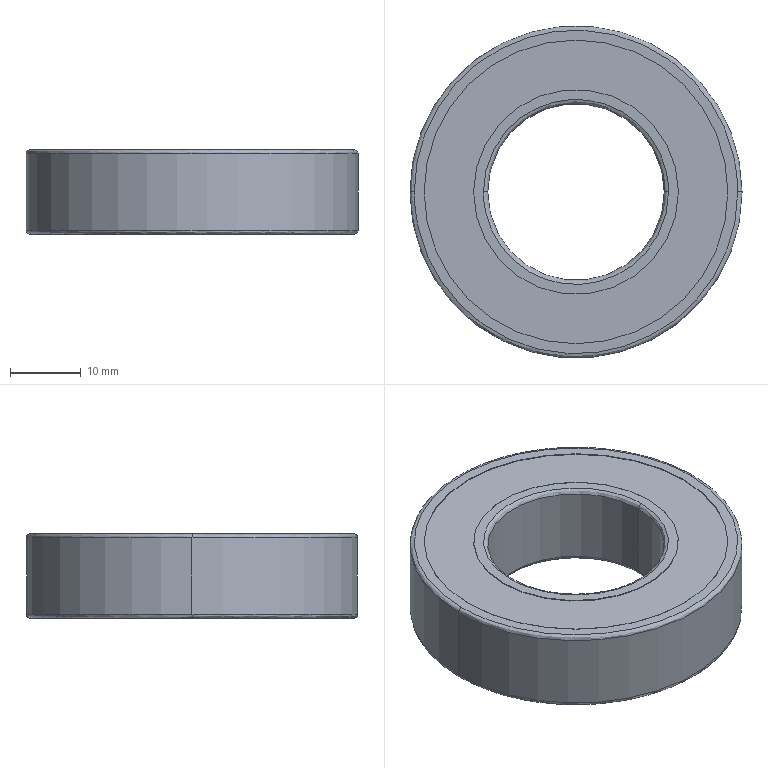Part | SolidWorks | features BaseBody 1 | 1 solid | 26 faces | box 47 x 47 x 12 mm | volume 14738 mm3 | cylinder 12 | spline 8 | plane 6 | commonest cylinder face diameters 29 x4 43 x4 25 x2 47 x2
STEP:
#1=CARTESIAN_POINT('',(-22.9,0.,-12.));
#2=VERTEX_POINT('',#1);
#3=CARTESIAN_POINT('',(22.9,0.,-12.));
#4=VERTEX_POINT('',#3);
#5=CARTESIAN_POINT('',(-22.9,0.,-12.));
#6=CARTESIAN_POINT('',(-22.9,-45.8,-12.));
#7=CARTESIAN_POINT('',(22.9,-45.8,-12.));
#8=CARTESIAN_POINT('',(22.9,0.,-12.));
#9=(BOUNDED_CURVE()B_SPLINE_CURVE(3,(#5,#6,#7,#8),.UNSPECIFIED.,.F.,.F.)B_SPLINE_CURVE_WITH_KNOTS((4,4),(0.,0.5),.UNSPECIFIED.)CURVE()GEOMETRIC_REPRESENTATION_ITEM()RATIONAL_B_SPLINE_CURVE((1.,0.3333,0.3333,1.))REPRESENTATION_ITEM(''));
#10=EDGE_CURVE('',#2,#4,#9,.T.);
#11=ORIENTED_EDGE('',*,*,#10,.T.);
#12=CARTESIAN_POINT('',(23.5,0.,-11.4));
#13=VERTEX_POINT('',#12);
#14=CARTESIAN_POINT('',(22.9,0.,-11.4));
#15=DIRECTION('',(0.,-1.,0.));
#16=DIRECTION('',(1.,0.,0.));
#17=AXIS2_PLACEMENT_3D('',#14,#15,#16);
#18=CIRCLE('',#17,0.6);
#19=EDGE_CURVE('',#4,#13,#18,.T.);
#20=ORIENTED_EDGE('',*,*,#19,.T.);
#21=CARTESIAN_POINT('',(-23.5,0.,-11.4));
#22=VERTEX_POINT('',#21);
#23=CARTESIAN_POINT('',(0.,0.,-11.4));
#24=DIRECTION('',(0.,0.,1.));
#25=DIRECTION('',(1.,0.,0.));
#26=AXIS2_PLACEMENT_3D('',#23,#24,#25);
#27=CIRCLE('',#26,23.5);
#28=EDGE_CURVE('',#22,#13,#27,.T.);
#29=ORIENTED_EDGE('',*,*,#28,.F.);
#30=CARTESIAN_POINT('',(-22.9,0.,-11.4));
#31=DIRECTION('',(0.,1.,0.));
#32=DIRECTION('',(-1.,0.,0.));
#33=AXIS2_PLACEMENT_3D('',#30,#31,#32);
#34=CIRCLE('',#33,0.6);
#35=EDGE_CURVE('',#2,#22,#34,.T.);
#36=ORIENTED_EDGE('',*,*,#35,.F.);
#37=EDGE_LOOP('',(#11,#20,#29,#36));
#38=FACE_OUTER_BOUND('',#37,.T.);
#39=CARTESIAN_POINT('',(22.9,0.,-12.));
#40=CARTESIAN_POINT('',(22.9,-45.8,-12.));
#41=CARTESIAN_POINT('',(-22.9,-45.8,-12.));
#42=CARTESIAN_POINT('',(-22.9,0.,-12.));
#43=CARTESIAN_POINT('',(23.251,0.,-12.));
#44=CARTESIAN_POINT('',(23.251,-46.503,-12.));
#45=CARTESIAN_POINT('',(-23.251,-46.503,-12.));
#46=CARTESIAN_POINT('',(-23.251,0.,-12.));
#47=CARTESIAN_POINT('',(23.5,0.,-11.751));
#48=CARTESIAN_POINT('',(23.5,-47.,-11.751));
#49=CARTESIAN_POINT('',(-23.5,-47.,-11.751));
#50=CARTESIAN_POINT('',(-23.5,0.,-11.751));
#51=CARTESIAN_POINT('',(23.5,0.,-11.4));
#52=CARTESIAN_POINT('',(23.5,-47.,-11.4));
#53=CARTESIAN_POINT('',(-23.5,-47.,-11.4));
#54=CARTESIAN_POINT('',(-23.5,0.,-11.4));
#55=(BOUNDED_SURFACE()B_SPLINE_SURFACE(3,3,((#39,#40,#41,#42),(#43,#44,#45,#46),(#47,#48,#49,#50),(#51,#52,#53,#54)),.UNSPECIFIED.,.F.,.F.,.F.)B_SPLINE_SURFACE_WITH_KNOTS((4,4),(4,4),(0.,1.),(0.,1.),.UNSPECIFIED.)GEOMETRIC_REPRESENTATION_ITEM()RATIONAL_B_SPLINE_SURFACE(((1.,0.3333,0.3333,1.),(0.8047,0.2682,0.2682,0.8047),(0.8047,0.2682,0.2682,0.8047),(1.,0.3333,0.3333,1.)))REPRESENTATION_ITEM('')SURFACE());
#56=ADVANCED_FACE('',(#38),#55,.T.);
#57=CARTESIAN_POINT('',(23.5,0.,-0.6));
#58=VERTEX_POINT('',#57);
#59=CARTESIAN_POINT('',(-23.5,0.,-0.6));
#60=VERTEX_POINT('',#59);
#61=CARTESIAN_POINT('',(0.,0.,-0.6));
#62=DIRECTION('',(0.,0.,-1.));
#63=DIRECTION('',(1.,0.,0.));
#64=AXIS2_PLACEMENT_3D('',#61,#62,#63);
#65=CIRCLE('',#64,23.5);
#66=EDGE_CURVE('',#58,#60,#65,.T.);
#67=ORIENTED_EDGE('',*,*,#66,.F.);
#68=CARTESIAN_POINT('',(22.9,0.,0.));
#69=VERTEX_POINT('',#68);
#70=CARTESIAN_POINT('',(22.9,0.,-0.6));
#71=DIRECTION('',(0.,-1.,0.));
#72=DIRECTION('',(1.,0.,0.));
#73=AXIS2_PLACEMENT_3D('',#70,#71,#72);
#74=CIRCLE('',#73,0.6);
#75=EDGE_CURVE('',#58,#69,#74,.T.);
#76=ORIENTED_EDGE('',*,*,#75,.T.);
#77=CARTESIAN_POINT('',(-22.9,0.,0.));
#78=VERTEX_POINT('',#77);
#79=CARTESIAN_POINT('',(22.9,0.,0.));
#80=CARTESIAN_POINT('',(22.9,-45.8,0.));
#81=CARTESIAN_POINT('',(-22.9,-45.8,0.));
#82=CARTESIAN_POINT('',(-22.9,0.,0.));
#83=(BOUNDED_CURVE()B_SPLINE_CURVE(3,(#79,#80,#81,#82),.UNSPECIFIED.,.F.,.F.)B_SPLINE_CURVE_WITH_KNOTS((4,4),(0.5,1.),.UNSPECIFIED.)CURVE()GEOMETRIC_REPRESENTATION_ITEM()RATIONAL_B_SPLINE_CURVE((1.,0.3333,0.3333,1.))REPRESENTATION_ITEM(''));
#84=EDGE_CURVE('',#69,#78,#83,.T.);
#85=ORIENTED_EDGE('',*,*,#84,.T.);
#86=CARTESIAN_POINT('',(-22.9,0.,-0.6));
#87=DIRECTION('',(0.,1.,0.));
#88=DIRECTION('',(-1.,0.,0.));
#89=AXIS2_PLACEMENT_3D('',#86,#87,#88);
#90=CIRCLE('',#89,0.6);
#91=EDGE_CURVE('',#60,#78,#90,.T.);
#92=ORIENTED_EDGE('',*,*,#91,.F.);
#93=EDGE_LOOP('',(#67,#76,#85,#92));
#94=FACE_OUTER_BOUND('',#93,.T.);
#95=CARTESIAN_POINT('',(23.5,0.,-0.6));
#96=CARTESIAN_POINT('',(23.5,-47.,-0.6));
#97=CARTESIAN_POINT('',(-23.5,-47.,-0.6));
#98=CARTESIAN_POINT('',(-23.5,0.,-0.6));
#99=CARTESIAN_POINT('',(23.5,0.,-0.2485));
#100=CARTESIAN_POINT('',(23.5,-47.,-0.2485));
#101=CARTESIAN_POINT('',(-23.5,-47.,-0.2485));
#102=CARTESIAN_POINT('',(-23.5,0.,-0.2485));
#103=CARTESIAN_POINT('',(23.251,0.,0.));
#104=CARTESIAN_POINT('',(23.251,-46.503,0.));
#105=CARTESIAN_POINT('',(-23.251,-46.503,0.));
#106=CARTESIAN_POINT('',(-23.251,0.,0.));
#107=CARTESIAN_POINT('',(22.9,0.,0.));
#108=CARTESIAN_POINT('',(22.9,-45.8,0.));
#109=CARTESIAN_POINT('',(-22.9,-45.8,0.));
#110=CARTESIAN_POINT('',(-22.9,0.,0.));
#111=(BOUNDED_SURFACE()B_SPLINE_SURFACE(3,3,((#95,#96,#97,#98),(#99,#100,#101,#102),(#103,#104,#105,#106),(#107,#108,#109,#110)),.UNSPECIFIED.,.F.,.F.,.F.)B_SPLINE_SURFACE_WITH_KNOTS((4,4),(4,4),(0.,1.),(0.,1.),.UNSPECIFIED.)GEOMETRIC_REPRESENTATION_ITEM()RATIONAL_B_SPLINE_SURFACE(((1.,0.3333,0.3333,1.),(0.8047,0.2682,0.2682,0.8047),(0.8047,0.2682,0.2682,0.8047),(1.,0.3333,0.3333,1.)))REPRESENTATION_ITEM('')SURFACE());
#112=ADVANCED_FACE('',(#94),#111,.T.);
#113=CARTESIAN_POINT('',(-12.5,0.,-11.4));
#114=VERTEX_POINT('',#113);
#115=CARTESIAN_POINT('',(12.5,0.,-11.4));
#116=VERTEX_POINT('',#115);
#117=CARTESIAN_POINT('',(0.,0.,-11.4));
#118=DIRECTION('',(0.,0.,1.));
#119=DIRECTION('',(-1.,0.,0.));
#120=AXIS2_PLACEMENT_3D('',#117,#118,#119);
#121=CIRCLE('',#120,12.5);
#122=EDGE_CURVE('',#114,#116,#121,.T.);
#123=ORIENTED_EDGE('',*,*,#122,.T.);
#124=CARTESIAN_POINT('',(13.1,0.,-12.));
#125=VERTEX_POINT('',#124);
#126=CARTESIAN_POINT('',(13.1,0.,-11.4));
#127=DIRECTION('',(0.,-1.,0.));
#128=DIRECTION('',(1.,0.,0.));
#129=AXIS2_PLACEMENT_3D('',#126,#127,#128);
#130=CIRCLE('',#129,0.6);
#131=EDGE_CURVE('',#116,#125,#130,.T.);
#132=ORIENTED_EDGE('',*,*,#131,.T.);
#133=CARTESIAN_POINT('',(-13.1,0.,-12.));
#134=VERTEX_POINT('',#133);
#135=CARTESIAN_POINT('',(-13.1,0.,-12.));
#136=CARTESIAN_POINT('',(-13.1,-0.4005,-12.));
#137=CARTESIAN_POINT('',(-13.073,-0.9989,-12.));
#138=CARTESIAN_POINT('',(-12.993,-1.693,-12.));
#139=CARTESIAN_POINT('',(-12.941,-2.039,-12.));
#140=CARTESIAN_POINT('',(-12.912,-2.211,-12.));
#141=CARTESIAN_POINT('',(-12.899,-2.285,-12.));
#142=CARTESIAN_POINT('',(-12.89,-2.334,-12.));
#143=CARTESIAN_POINT('',(-12.886,-2.358,-12.));
#144=CARTESIAN_POINT('',(-12.804,-2.801,-12.));
#145=CARTESIAN_POINT('',(-12.658,-3.419,-12.));
#146=CARTESIAN_POINT('',(-12.437,-4.126,-12.));
#147=CARTESIAN_POINT('',(-12.313,-4.475,-12.));
#148=CARTESIAN_POINT('',(-12.257,-4.624,-12.));
#149=CARTESIAN_POINT('',(-12.219,-4.723,-12.));
#150=CARTESIAN_POINT('',(-12.201,-4.771,-12.));
#151=CARTESIAN_POINT('',(-12.017,-5.233,-12.));
#152=CARTESIAN_POINT('',(-11.743,-5.835,-12.));
#153=CARTESIAN_POINT('',(-11.371,-6.511,-12.));
#154=CARTESIAN_POINT('',(-11.172,-6.842,-12.));
#155=CARTESIAN_POINT('',(-11.084,-6.982,-12.));
#156=CARTESIAN_POINT('',(-11.025,-7.076,-12.));
#157=CARTESIAN_POINT('',(-10.996,-7.121,-12.));
#158=CARTESIAN_POINT('',(-10.47,-7.925,-12.));
#159=CARTESIAN_POINT('',(-9.902,-8.624,-12.));
#160=CARTESIAN_POINT('',(-8.943,-9.583,-12.));
#161=CARTESIAN_POINT('',(-8.442,-10.035,-12.));
#162=CARTESIAN_POINT('',(-7.818,-10.516,-12.));
#163=CARTESIAN_POINT('',(-7.497,-10.744,-12.));
#164=CARTESIAN_POINT('',(-7.357,-10.839,-12.));
#165=CARTESIAN_POINT('',(-7.263,-10.902,-12.));
#166=CARTESIAN_POINT('',(-7.215,-10.934,-12.));
#167=CARTESIAN_POINT('',(-6.798,-11.207,-12.));
#168=CARTESIAN_POINT('',(-6.227,-11.54,-12.));
#169=CARTESIAN_POINT('',(-5.534,-11.878,-12.));
#170=CARTESIAN_POINT('',(-5.18,-12.033,-12.));
#171=CARTESIAN_POINT('',(-5.002,-12.108,-12.));
#172=CARTESIAN_POINT('',(-4.925,-12.139,-12.));
#173=CARTESIAN_POINT('',(-4.873,-12.16,-12.));
#174=CARTESIAN_POINT('',(-4.847,-12.17,-12.));
#175=CARTESIAN_POINT('',(-4.427,-12.337,-12.));
#176=CARTESIAN_POINT('',(-3.826,-12.541,-12.));
#177=CARTESIAN_POINT('',(-3.11,-12.729,-12.));
#178=CARTESIAN_POINT('',(-2.748,-12.809,-12.));
#179=CARTESIAN_POINT('',(-2.566,-12.846,-12.));
#180=CARTESIAN_POINT('',(-2.488,-12.862,-12.));
#181=CARTESIAN_POINT('',(-2.436,-12.872,-12.));
#182=CARTESIAN_POINT('',(-2.408,-12.877,-12.));
#183=CARTESIAN_POINT('',(-1.596,-13.027,-12.));
#184=CARTESIAN_POINT('',(-0.8009,-13.1,-12.));
#185=CARTESIAN_POINT('',(0.4005,-13.1,-12.));
#186=CARTESIAN_POINT('',(0.9988,-13.073,-12.));
#187=CARTESIAN_POINT('',(1.693,-12.993,-12.));
#188=CARTESIAN_POINT('',(2.039,-12.941,-12.));
#189=CARTESIAN_POINT('',(2.211,-12.912,-12.));
#190=CARTESIAN_POINT('',(2.285,-12.899,-12.));
#191=CARTESIAN_POINT('',(2.334,-12.89,-12.));
#192=CARTESIAN_POINT('',(2.358,-12.886,-12.));
#193=CARTESIAN_POINT('',(2.801,-12.804,-12.));
#194=CARTESIAN_POINT('',(3.419,-12.658,-12.));
#195=CARTESIAN_POINT('',(4.126,-12.437,-12.));
#196=CARTESIAN_POINT('',(4.475,-12.313,-12.));
#197=CARTESIAN_POINT('',(4.624,-12.257,-12.));
#198=CARTESIAN_POINT('',(4.723,-12.219,-12.));
#199=CARTESIAN_POINT('',(4.771,-12.201,-12.));
#200=CARTESIAN_POINT('',(5.233,-12.017,-12.));
#201=CARTESIAN_POINT('',(5.835,-11.743,-12.));
#202=CARTESIAN_POINT('',(6.511,-11.371,-12.));
#203=CARTESIAN_POINT('',(6.842,-11.172,-12.));
#204=CARTESIAN_POINT('',(6.982,-11.084,-12.));
#205=CARTESIAN_POINT('',(7.076,-11.025,-12.));
#206=CARTESIAN_POINT('',(7.121,-10.996,-12.));
#207=CARTESIAN_POINT('',(7.925,-10.47,-12.));
#208=CARTESIAN_POINT('',(8.624,-9.902,-12.));
#209=CARTESIAN_POINT('',(9.583,-8.943,-12.));
#210=CARTESIAN_POINT('',(10.035,-8.442,-12.));
#211=CARTESIAN_POINT('',(10.516,-7.818,-12.));
#212=CARTESIAN_POINT('',(10.744,-7.497,-12.));
#213=CARTESIAN_POINT('',(10.839,-7.357,-12.));
#214=CARTESIAN_POINT('',(10.902,-7.263,-12.));
#215=CARTESIAN_POINT('',(10.934,-7.215,-12.));
#216=CARTESIAN_POINT('',(11.207,-6.798,-12.));
#217=CARTESIAN_POINT('',(11.54,-6.227,-12.));
#218=CARTESIAN_POINT('',(11.878,-5.534,-12.));
#219=CARTESIAN_POINT('',(12.033,-5.18,-12.));
#220=CARTESIAN_POINT('',(12.108,-5.002,-12.));
#221=CARTESIAN_POINT('',(12.139,-4.925,-12.));
#222=CARTESIAN_POINT('',(12.16,-4.873,-12.));
#223=CARTESIAN_POINT('',(12.17,-4.847,-12.));
#224=CARTESIAN_POINT('',(12.337,-4.427,-12.));
#225=CARTESIAN_POINT('',(12.541,-3.826,-12.));
#226=CARTESIAN_POINT('',(12.729,-3.11,-12.));
#227=CARTESIAN_POINT('',(12.809,-2.748,-12.));
#228=CARTESIAN_POINT('',(12.846,-2.566,-12.));
#229=CARTESIAN_POINT('',(12.862,-2.488,-12.));
#230=CARTESIAN_POINT('',(12.872,-2.436,-12.));
#231=CARTESIAN_POINT('',(12.877,-2.408,-12.));
#232=CARTESIAN_POINT('',(13.027,-1.596,-12.));
#233=CARTESIAN_POINT('',(13.1,-0.8009,-12.));
#234=CARTESIAN_POINT('',(13.1,0.,-12.));
#235=B_SPLINE_CURVE_WITH_KNOTS('',3,(#135,#136,#137,#138,#139,#140,#141,#142,#143,#144,#145,#146,#147,#148,#149,#150,#151,#152,#153,#154,#155,#156,#157,#158,#159,#160,#161,#162,#163,#164,#165,#166,#167,#168,#169,#170,#171,#172,#173,#174,#175,#176,#177,#178,#179,#180,#181,#182,#183,#184,#185,#186,#187,#188,#189,#190,#191,#192,#193,#194,#195,#196,#197,#198,#199,#200,#201,#202,#203,#204,#205,#206,#207,#208,#209,#210,#211,#212,#213,#214,#215,#216,#217,#218,#219,#220,#221,#222,#223,#224,#225,#226,#227,#228,#229,#230,#231,#232,#233,#234),.UNSPECIFIED.,.F.,.F.,(4,1,1,1,1,2,2,1,1,1,2,2,1,1,1,2,2,2,1,1,1,2,2,1,1,1,1,2,2,1,1,1,1,2,2,2,1,1,1,1,2,2,1,1,1,2,2,1,1,1,2,2,2,1,1,1,2,2,1,1,1,1,2,2,1,1,1,1,2,2,4),(0.,0.01563,0.02344,0.02734,0.0293,0.03027,0.03125,0.04688,0.05469,0.05859,0.06055,0.0625,0.07813,0.08594,0.08984,0.0918,0.09375,0.125,0.1406,0.1484,0.1523,0.1543,0.1563,0.1719,0.1797,0.1836,0.1855,0.1865,0.1875,0.2031,0.2109,0.2148,0.2168,0.2178,0.2188,0.25,0.2656,0.2734,0.2773,0.2793,0.2803,0.2813,0.2969,0.3047,0.3086,0.3105,0.3125,0.3281,0.3359,0.3398,0.3418,0.3438,0.375,0.3906,0.3984,0.4023,0.4043,0.4063,0.4219,0.4297,0.4336,0.4355,0.4365,0.4375,0.4531,0.4609,0.4648,0.4668,0.4678,0.4688,0.5),.UNSPECIFIED.);
#236=EDGE_CURVE('',#134,#125,#235,.T.);
#237=ORIENTED_EDGE('',*,*,#236,.F.);
#238=CARTESIAN_POINT('',(-13.1,0.,-11.4));
#239=DIRECTION('',(0.,1.,0.));
#240=DIRECTION('',(-1.,0.,0.));
#241=AXIS2_PLACEMENT_3D('',#238,#239,#240);
#242=CIRCLE('',#241,0.6);
#243=EDGE_CURVE('',#114,#134,#242,.T.);
#244=ORIENTED_EDGE('',*,*,#243,.F.);
#245=EDGE_LOOP('',(#123,#132,#237,#244));
#246=FACE_OUTER_BOUND('',#245,.T.);
#247=CARTESIAN_POINT('',(12.5,0.,-11.4));
#248=CARTESIAN_POINT('',(12.5,-25.,-11.4));
#249=CARTESIAN_POINT('',(-12.5,-25.,-11.4));
#250=CARTESIAN_POINT('',(-12.5,0.,-11.4));
#251=CARTESIAN_POINT('',(12.5,0.,-11.751));
#252=CARTESIAN_POINT('',(12.5,-25.,-11.751));
#253=CARTESIAN_POINT('',(-12.5,-25.,-11.751));
#254=CARTESIAN_POINT('',(-12.5,0.,-11.751));
#255=CARTESIAN_POINT('',(12.749,0.,-12.));
#256=CARTESIAN_POINT('',(12.749,-25.497,-12.));
#257=CARTESIAN_POINT('',(-12.749,-25.497,-12.));
#258=CARTESIAN_POINT('',(-12.749,0.,-12.));
#259=CARTESIAN_POINT('',(13.1,0.,-12.));
#260=CARTESIAN_POINT('',(13.1,-26.2,-12.));
#261=CARTESIAN_POINT('',(-13.1,-26.2,-12.));
#262=CARTESIAN_POINT('',(-13.1,0.,-12.));
#263=(BOUNDED_SURFACE()B_SPLINE_SURFACE(3,3,((#247,#248,#249,#250),(#251,#252,#253,#254),(#255,#256,#257,#258),(#259,#260,#261,#262)),.UNSPECIFIED.,.F.,.F.,.F.)B_SPLINE_SURFACE_WITH_KNOTS((4,4),(4,4),(0.,1.),(0.,1.),.UNSPECIFIED.)GEOMETRIC_REPRESENTATION_ITEM()RATIONAL_B_SPLINE_SURFACE(((1.,0.3333,0.3333,1.),(0.8047,0.2682,0.2682,0.8047),(0.8047,0.2682,0.2682,0.8047),(1.,0.3333,0.3333,1.)))REPRESENTATION_ITEM('')SURFACE());
#264=ADVANCED_FACE('',(#246),#263,.T.);
#265=CARTESIAN_POINT('',(13.1,0.,0.));
#266=VERTEX_POINT('',#265);
#267=CARTESIAN_POINT('',(-13.1,0.,0.));
#268=VERTEX_POINT('',#267);
#269=CARTESIAN_POINT('',(13.1,0.,0.));
#270=CARTESIAN_POINT('',(13.1,-0.4005,0.));
#271=CARTESIAN_POINT('',(13.073,-0.9988,0.));
#272=CARTESIAN_POINT('',(12.993,-1.693,0.));
#273=CARTESIAN_POINT('',(12.941,-2.039,0.));
#274=CARTESIAN_POINT('',(12.912,-2.211,0.));
#275=CARTESIAN_POINT('',(12.899,-2.285,0.));
#276=CARTESIAN_POINT('',(12.89,-2.334,0.));
#277=CARTESIAN_POINT('',(12.886,-2.358,0.));
#278=CARTESIAN_POINT('',(12.804,-2.801,0.));
#279=CARTESIAN_POINT('',(12.658,-3.419,0.));
#280=CARTESIAN_POINT('',(12.437,-4.126,0.));
#281=CARTESIAN_POINT('',(12.313,-4.475,0.));
#282=CARTESIAN_POINT('',(12.257,-4.624,0.));
#283=CARTESIAN_POINT('',(12.219,-4.723,0.));
#284=CARTESIAN_POINT('',(12.201,-4.771,0.));
#285=CARTESIAN_POINT('',(12.017,-5.233,0.));
#286=CARTESIAN_POINT('',(11.743,-5.835,0.));
#287=CARTESIAN_POINT('',(11.371,-6.511,0.));
#288=CARTESIAN_POINT('',(11.172,-6.842,0.));
#289=CARTESIAN_POINT('',(11.084,-6.982,0.));
#290=CARTESIAN_POINT('',(11.025,-7.076,0.));
#291=CARTESIAN_POINT('',(10.996,-7.121,0.));
#292=CARTESIAN_POINT('',(10.47,-7.925,0.));
#293=CARTESIAN_POINT('',(9.902,-8.624,0.));
#294=CARTESIAN_POINT('',(8.943,-9.583,0.));
#295=CARTESIAN_POINT('',(8.442,-10.035,0.));
#296=CARTESIAN_POINT('',(7.818,-10.516,0.));
#297=CARTESIAN_POINT('',(7.497,-10.744,0.));
#298=CARTESIAN_POINT('',(7.357,-10.839,0.));
#299=CARTESIAN_POINT('',(7.263,-10.902,0.));
#300=CARTESIAN_POINT('',(7.215,-10.934,0.));
#301=CARTESIAN_POINT('',(6.798,-11.207,0.));
#302=CARTESIAN_POINT('',(6.227,-11.54,0.));
#303=CARTESIAN_POINT('',(5.534,-11.878,0.));
#304=CARTESIAN_POINT('',(5.18,-12.033,0.));
#305=CARTESIAN_POINT('',(5.002,-12.108,0.));
#306=CARTESIAN_POINT('',(4.925,-12.139,0.));
#307=CARTESIAN_POINT('',(4.873,-12.16,0.));
#308=CARTESIAN_POINT('',(4.847,-12.17,0.));
#309=CARTESIAN_POINT('',(4.427,-12.337,0.));
#310=CARTESIAN_POINT('',(3.826,-12.541,0.));
#311=CARTESIAN_POINT('',(3.11,-12.729,0.));
#312=CARTESIAN_POINT('',(2.748,-12.809,0.));
#313=CARTESIAN_POINT('',(2.566,-12.846,0.));
#314=CARTESIAN_POINT('',(2.488,-12.862,0.));
#315=CARTESIAN_POINT('',(2.436,-12.872,0.));
#316=CARTESIAN_POINT('',(2.408,-12.877,0.));
#317=CARTESIAN_POINT('',(1.596,-13.027,0.));
#318=CARTESIAN_POINT('',(0.8009,-13.1,0.));
#319=CARTESIAN_POINT('',(-0.4005,-13.1,0.));
#320=CARTESIAN_POINT('',(-0.9988,-13.073,0.));
#321=CARTESIAN_POINT('',(-1.693,-12.993,0.));
#322=CARTESIAN_POINT('',(-2.039,-12.941,0.));
#323=CARTESIAN_POINT('',(-2.211,-12.912,0.));
#324=CARTESIAN_POINT('',(-2.285,-12.899,0.));
#325=CARTESIAN_POINT('',(-2.334,-12.89,0.));
#326=CARTESIAN_POINT('',(-2.358,-12.886,0.));
#327=CARTESIAN_POINT('',(-2.801,-12.804,0.));
#328=CARTESIAN_POINT('',(-3.419,-12.658,0.));
#329=CARTESIAN_POINT('',(-4.126,-12.437,0.));
#330=CARTESIAN_POINT('',(-4.475,-12.313,0.));
#331=CARTESIAN_POINT('',(-4.624,-12.257,0.));
#332=CARTESIAN_POINT('',(-4.723,-12.219,0.));
#333=CARTESIAN_POINT('',(-4.771,-12.201,0.));
#334=CARTESIAN_POINT('',(-5.233,-12.017,0.));
#335=CARTESIAN_POINT('',(-5.835,-11.743,0.));
#336=CARTESIAN_POINT('',(-6.511,-11.371,0.));
#337=CARTESIAN_POINT('',(-6.842,-11.172,0.));
#338=CARTESIAN_POINT('',(-6.982,-11.084,0.));
#339=CARTESIAN_POINT('',(-7.076,-11.025,0.));
#340=CARTESIAN_POINT('',(-7.121,-10.996,0.));
#341=CARTESIAN_POINT('',(-7.925,-10.47,0.));
#342=CARTESIAN_POINT('',(-8.624,-9.902,0.));
#343=CARTESIAN_POINT('',(-9.583,-8.943,0.));
#344=CARTESIAN_POINT('',(-10.035,-8.442,0.));
#345=CARTESIAN_POINT('',(-10.516,-7.818,0.));
#346=CARTESIAN_POINT('',(-10.744,-7.497,0.));
#347=CARTESIAN_POINT('',(-10.839,-7.357,0.));
#348=CARTESIAN_POINT('',(-10.902,-7.263,0.));
#349=CARTESIAN_POINT('',(-10.934,-7.215,0.));
#350=CARTESIAN_POINT('',(-11.207,-6.798,0.));
#351=CARTESIAN_POINT('',(-11.54,-6.227,0.));
#352=CARTESIAN_POINT('',(-11.878,-5.534,0.));
#353=CARTESIAN_POINT('',(-12.033,-5.18,0.));
#354=CARTESIAN_POINT('',(-12.108,-5.002,0.));
#355=CARTESIAN_POINT('',(-12.139,-4.925,0.));
#356=CARTESIAN_POINT('',(-12.16,-4.873,0.));
#357=CARTESIAN_POINT('',(-12.17,-4.847,0.));
#358=CARTESIAN_POINT('',(-12.337,-4.427,0.));
#359=CARTESIAN_POINT('',(-12.541,-3.826,0.));
#360=CARTESIAN_POINT('',(-12.729,-3.11,0.));
#361=CARTESIAN_POINT('',(-12.809,-2.748,0.));
#362=CARTESIAN_POINT('',(-12.846,-2.566,0.));
#363=CARTESIAN_POINT('',(-12.862,-2.488,0.));
#364=CARTESIAN_POINT('',(-12.872,-2.436,0.));
#365=CARTESIAN_POINT('',(-12.877,-2.408,0.));
#366=CARTESIAN_POINT('',(-13.027,-1.596,0.));
#367=CARTESIAN_POINT('',(-13.1,-0.8014,0.));
#368=CARTESIAN_POINT('',(-13.1,0.,0.));
#369=B_SPLINE_CURVE_WITH_KNOTS('',3,(#269,#270,#271,#272,#273,#274,#275,#276,#277,#278,#279,#280,#281,#282,#283,#284,#285,#286,#287,#288,#289,#290,#291,#292,#293,#294,#295,#296,#297,#298,#299,#300,#301,#302,#303,#304,#305,#306,#307,#308,#309,#310,#311,#312,#313,#314,#315,#316,#317,#318,#319,#320,#321,#322,#323,#324,#325,#326,#327,#328,#329,#330,#331,#332,#333,#334,#335,#336,#337,#338,#339,#340,#341,#342,#343,#344,#345,#346,#347,#348,#349,#350,#351,#352,#353,#354,#355,#356,#357,#358,#359,#360,#361,#362,#363,#364,#365,#366,#367,#368),.UNSPECIFIED.,.F.,.F.,(4,1,1,1,1,2,2,1,1,1,2,2,1,1,1,2,2,2,1,1,1,2,2,1,1,1,1,2,2,1,1,1,1,2,2,2,1,1,1,1,2,2,1,1,1,2,2,1,1,1,2,2,2,1,1,1,2,2,1,1,1,1,2,2,1,1,1,1,2,2,4),(0.5,0.5156,0.5234,0.5273,0.5293,0.5303,0.5313,0.5469,0.5547,0.5586,0.5605,0.5625,0.5781,0.5859,0.5898,0.5918,0.5938,0.625,0.6406,0.6484,0.6523,0.6543,0.6563,0.6719,0.6797,0.6836,0.6855,0.6865,0.6875,0.7031,0.7109,0.7148,0.7168,0.7178,0.7188,0.75,0.7656,0.7734,0.7773,0.7793,0.7803,0.7813,0.7969,0.8047,0.8086,0.8105,0.8125,0.8281,0.8359,0.8398,0.8418,0.8438,0.875,0.8906,0.8984,0.9023,0.9043,0.9062,0.9219,0.9297,0.9336,0.9355,0.9365,0.9375,0.9531,0.9609,0.9648,0.9668,0.9678,0.9687,1.),.UNSPECIFIED.);
#370=EDGE_CURVE('',#266,#268,#369,.T.);
#371=ORIENTED_EDGE('',*,*,#370,.F.);
#372=CARTESIAN_POINT('',(12.5,0.,-0.6));
#373=VERTEX_POINT('',#372);
#374=CARTESIAN_POINT('',(13.1,0.,-0.6));
#375=DIRECTION('',(0.,-1.,0.));
#376=DIRECTION('',(1.,0.,0.));
#377=AXIS2_PLACEMENT_3D('',#374,#375,#376);
#378=CIRCLE('',#377,0.6);
#379=EDGE_CURVE('',#266,#373,#378,.T.);
#380=ORIENTED_EDGE('',*,*,#379,.T.);
#381=CARTESIAN_POINT('',(-12.5,0.,-0.6));
#382=VERTEX_POINT('',#381);
#383=CARTESIAN_POINT('',(0.,0.,-0.6));
#384=DIRECTION('',(0.,0.,-1.));
#385=DIRECTION('',(-1.,0.,0.));
#386=AXIS2_PLACEMENT_3D('',#383,#384,#385);
#387=CIRCLE('',#386,12.5);
#388=EDGE_CURVE('',#373,#382,#387,.T.);
#389=ORIENTED_EDGE('',*,*,#388,.T.);
#390=CARTESIAN_POINT('',(-13.1,0.,-0.6));
#391=DIRECTION('',(0.,1.,0.));
#392=DIRECTION('',(-1.,0.,0.));
#393=AXIS2_PLACEMENT_3D('',#390,#391,#392);
#394=CIRCLE('',#393,0.6);
#395=EDGE_CURVE('',#268,#382,#394,.T.);
#396=ORIENTED_EDGE('',*,*,#395,.F.);
#397=EDGE_LOOP('',(#371,#380,#389,#396));
#398=FACE_OUTER_BOUND('',#397,.T.);
#399=CARTESIAN_POINT('',(13.1,0.,0.));
#400=CARTESIAN_POINT('',(13.1,-26.2,0.));
#401=CARTESIAN_POINT('',(-13.1,-26.2,0.));
#402=CARTESIAN_POINT('',(-13.1,0.,0.));
#403=CARTESIAN_POINT('',(12.749,0.,0.));
#404=CARTESIAN_POINT('',(12.749,-25.497,0.));
#405=CARTESIAN_POINT('',(-12.749,-25.497,0.));
#406=CARTESIAN_POINT('',(-12.749,0.,0.));
#407=CARTESIAN_POINT('',(12.5,0.,-0.2485));
#408=CARTESIAN_POINT('',(12.5,-25.,-0.2485));
#409=CARTESIAN_POINT('',(-12.5,-25.,-0.2485));
#410=CARTESIAN_POINT('',(-12.5,0.,-0.2485));
#411=CARTESIAN_POINT('',(12.5,0.,-0.6));
#412=CARTESIAN_POINT('',(12.5,-25.,-0.6));
#413=CARTESIAN_POINT('',(-12.5,-25.,-0.6));
#414=CARTESIAN_POINT('',(-12.5,0.,-0.6));
#415=(BOUNDED_SURFACE()B_SPLINE_SURFACE(3,3,((#399,#400,#401,#402),(#403,#404,#405,#406),(#407,#408,#409,#410),(#411,#412,#413,#414)),.UNSPECIFIED.,.F.,.F.,.F.)B_SPLINE_SURFACE_WITH_KNOTS((4,4),(4,4),(0.,1.),(0.,1.),.UNSPECIFIED.)GEOMETRIC_REPRESENTATION_ITEM()RATIONAL_B_SPLINE_SURFACE(((1.,0.3333,0.3333,1.),(0.8047,0.2682,0.2682,0.8047),(0.8047,0.2682,0.2682,0.8047),(1.,0.3333,0.3333,1.)))REPRESENTATION_ITEM('')SURFACE());
#416=ADVANCED_FACE('',(#398),#415,.T.);
#417=CARTESIAN_POINT('',(0.,0.,-11.4));
#418=DIRECTION('',(0.,0.,1.));
#419=DIRECTION('',(1.,0.,0.));
#420=AXIS2_PLACEMENT_3D('',#417,#418,#419);
#421=CIRCLE('',#420,23.5);
#422=EDGE_CURVE('',#13,#22,#421,.T.);
#423=ORIENTED_EDGE('',*,*,#422,.T.);
#424=CARTESIAN_POINT('',(-23.5,0.,-12.));
#425=DIRECTION('',(0.,0.,1.));
#426=VECTOR('',#425,1000.);
#427=LINE('',#424,#426);
#428=EDGE_CURVE('',#22,#60,#427,.T.);
#429=ORIENTED_EDGE('',*,*,#428,.T.);
#430=CARTESIAN_POINT('',(0.,0.,-0.6));
#431=DIRECTION('',(0.,0.,-1.));
#432=DIRECTION('',(1.,0.,0.));
#433=AXIS2_PLACEMENT_3D('',#430,#431,#432);
#434=CIRCLE('',#433,23.5);
#435=EDGE_CURVE('',#60,#58,#434,.T.);
#436=ORIENTED_EDGE('',*,*,#435,.T.);
#437=CARTESIAN_POINT('',(23.5,0.,-12.));
#438=DIRECTION('',(0.,0.,1.));
#439=VECTOR('',#438,1000.);
#440=LINE('',#437,#439);
#441=EDGE_CURVE('',#13,#58,#440,.T.);
#442=ORIENTED_EDGE('',*,*,#441,.F.);
#443=EDGE_LOOP('',(#423,#429,#436,#442));
#444=FACE_OUTER_BOUND('',#443,.T.);
#445=CARTESIAN_POINT('',(0.,0.,-12.));
#446=DIRECTION('',(0.,0.,1.));
#447=DIRECTION('',(1.,0.,0.));
#448=AXIS2_PLACEMENT_3D('',#445,#446,#447);
#449=CYLINDRICAL_SURFACE('',#448,23.5);
#450=ADVANCED_FACE('',(#444),#449,.T.);
#451=CARTESIAN_POINT('',(-21.5,0.,-12.));
#452=VERTEX_POINT('',#451);
#453=CARTESIAN_POINT('',(21.5,0.,-12.));
#454=VERTEX_POINT('',#453);
#455=CARTESIAN_POINT('',(0.,0.,-12.));
#456=DIRECTION('',(0.,0.,1.));
#457=DIRECTION('',(1.,0.,0.));
#458=AXIS2_PLACEMENT_3D('',#455,#456,#457);
#459=CIRCLE('',#458,21.5);
#460=EDGE_CURVE('',#452,#454,#459,.T.);
#461=ORIENTED_EDGE('',*,*,#460,.F.);
#462=CARTESIAN_POINT('',(-21.5,0.,-11.9));
#463=VERTEX_POINT('',#462);
#464=CARTESIAN_POINT('',(-21.5,0.,-12.));
#465=DIRECTION('',(0.,0.,1.));
#466=VECTOR('',#465,1000.);
#467=LINE('',#464,#466);
#468=EDGE_CURVE('',#452,#463,#467,.T.);
#469=ORIENTED_EDGE('',*,*,#468,.T.);
#470=CARTESIAN_POINT('',(21.5,0.,-11.9));
#471=VERTEX_POINT('',#470);
#472=CARTESIAN_POINT('',(0.,0.,-11.9));
#473=DIRECTION('',(0.,0.,-1.));
#474=DIRECTION('',(1.,0.,0.));
#475=AXIS2_PLACEMENT_3D('',#472,#473,#474);
#476=CIRCLE('',#475,21.5);
#477=EDGE_CURVE('',#471,#463,#476,.T.);
#478=ORIENTED_EDGE('',*,*,#477,.F.);
#479=CARTESIAN_POINT('',(21.5,0.,-12.));
#480=DIRECTION('',(0.,0.,1.));
#481=VECTOR('',#480,1000.);
#482=LINE('',#479,#481);
#483=EDGE_CURVE('',#454,#471,#482,.T.);
#484=ORIENTED_EDGE('',*,*,#483,.F.);
#485=EDGE_LOOP('',(#461,#469,#478,#484));
#486=FACE_OUTER_BOUND('',#485,.T.);
#487=CARTESIAN_POINT('',(0.,0.,-12.));
#488=DIRECTION('',(0.,0.,1.));
#489=DIRECTION('',(1.,0.,0.));
#490=AXIS2_PLACEMENT_3D('',#487,#488,#489);
#491=CYLINDRICAL_SURFACE('',#490,21.5);
#492=ADVANCED_FACE('',(#486),#491,.F.);
#493=CARTESIAN_POINT('',(-21.5,0.,-0.1));
#494=VERTEX_POINT('',#493);
#495=CARTESIAN_POINT('',(21.5,0.,-0.1));
#496=VERTEX_POINT('',#495);
#497=CARTESIAN_POINT('',(0.,0.,-0.1));
#498=DIRECTION('',(0.,0.,1.));
#499=DIRECTION('',(1.,0.,0.));
#500=AXIS2_PLACEMENT_3D('',#497,#498,#499);
#501=CIRCLE('',#500,21.5);
#502=EDGE_CURVE('',#494,#496,#501,.T.);
#503=ORIENTED_EDGE('',*,*,#502,.F.);
#504=CARTESIAN_POINT('',(-21.5,0.,0.));
#505=VERTEX_POINT('',#504);
#506=CARTESIAN_POINT('',(-21.5,0.,-12.));
#507=DIRECTION('',(0.,0.,1.));
#508=VECTOR('',#507,1000.);
#509=LINE('',#506,#508);
#510=EDGE_CURVE('',#494,#505,#509,.T.);
#511=ORIENTED_EDGE('',*,*,#510,.T.);
#512=CARTESIAN_POINT('',(21.5,0.,0.));
#513=VERTEX_POINT('',#512);
#514=CARTESIAN_POINT('',(0.,0.,0.));
#515=DIRECTION('',(0.,0.,-1.));
#516=DIRECTION('',(1.,0.,0.));
#517=AXIS2_PLACEMENT_3D('',#514,#515,#516);
#518=CIRCLE('',#517,21.5);
#519=EDGE_CURVE('',#513,#505,#518,.T.);
#520=ORIENTED_EDGE('',*,*,#519,.F.);
#521=CARTESIAN_POINT('',(21.5,0.,-12.));
#522=DIRECTION('',(0.,0.,1.));
#523=VECTOR('',#522,1000.);
#524=LINE('',#521,#523);
#525=EDGE_CURVE('',#496,#513,#524,.T.);
#526=ORIENTED_EDGE('',*,*,#525,.F.);
#527=EDGE_LOOP('',(#503,#511,#520,#526));
#528=FACE_OUTER_BOUND('',#527,.T.);
#529=CARTESIAN_POINT('',(0.,0.,-12.));
#530=DIRECTION('',(0.,0.,1.));
#531=DIRECTION('',(1.,0.,0.));
#532=AXIS2_PLACEMENT_3D('',#529,#530,#531);
#533=CYLINDRICAL_SURFACE('',#532,21.5);
#534=ADVANCED_FACE('',(#528),#533,.F.);
#535=CARTESIAN_POINT('',(14.5,0.,-12.));
#536=VERTEX_POINT('',#535);
#537=CARTESIAN_POINT('',(-14.5,0.,-12.));
#538=VERTEX_POINT('',#537);
#539=CARTESIAN_POINT('',(0.,0.,-12.));
#540=DIRECTION('',(0.,0.,1.));
#541=DIRECTION('',(1.,0.,0.));
#542=AXIS2_PLACEMENT_3D('',#539,#540,#541);
#543=CIRCLE('',#542,14.5);
#544=EDGE_CURVE('',#536,#538,#543,.T.);
#545=ORIENTED_EDGE('',*,*,#544,.T.);
#546=CARTESIAN_POINT('',(-14.5,0.,-11.9));
#547=VERTEX_POINT('',#546);
#548=CARTESIAN_POINT('',(-14.5,0.,-12.));
#549=DIRECTION('',(0.,0.,1.));
#550=VECTOR('',#549,1000.);
#551=LINE('',#548,#550);
#552=EDGE_CURVE('',#538,#547,#551,.T.);
#553=ORIENTED_EDGE('',*,*,#552,.T.);
#554=CARTESIAN_POINT('',(14.5,0.,-11.9));
#555=VERTEX_POINT('',#554);
#556=CARTESIAN_POINT('',(0.,0.,-11.9));
#557=DIRECTION('',(0.,0.,1.));
#558=DIRECTION('',(1.,0.,0.));
#559=AXIS2_PLACEMENT_3D('',#556,#557,#558);
#560=CIRCLE('',#559,14.5);
#561=EDGE_CURVE('',#555,#547,#560,.T.);
#562=ORIENTED_EDGE('',*,*,#561,.F.);
#563=CARTESIAN_POINT('',(14.5,0.,-12.));
#564=DIRECTION('',(0.,0.,1.));
#565=VECTOR('',#564,1000.);
#566=LINE('',#563,#565);
#567=EDGE_CURVE('',#536,#555,#566,.T.);
#568=ORIENTED_EDGE('',*,*,#567,.F.);
#569=EDGE_LOOP('',(#545,#553,#562,#568));
#570=FACE_OUTER_BOUND('',#569,.T.);
#571=CARTESIAN_POINT('',(0.,0.,-12.));
#572=DIRECTION('',(0.,0.,1.));
#573=DIRECTION('',(1.,0.,0.));
#574=AXIS2_PLACEMENT_3D('',#571,#572,#573);
#575=CYLINDRICAL_SURFACE('',#574,14.5);
#576=ADVANCED_FACE('',(#570),#575,.T.);
#577=CARTESIAN_POINT('',(-14.5,0.,-0.1));
#578=VERTEX_POINT('',#577);
#579=CARTESIAN_POINT('',(14.5,0.,-0.1));
#580=VERTEX_POINT('',#579);
#581=CARTESIAN_POINT('',(0.,0.,-0.1));
#582=DIRECTION('',(0.,0.,-1.));
#583=DIRECTION('',(1.,0.,0.));
#584=AXIS2_PLACEMENT_3D('',#581,#582,#583);
#585=CIRCLE('',#584,14.5);
#586=EDGE_CURVE('',#578,#580,#585,.T.);
#587=ORIENTED_EDGE('',*,*,#586,.F.);
#588=CARTESIAN_POINT('',(-14.5,0.,0.));
#589=VERTEX_POINT('',#588);
#590=CARTESIAN_POINT('',(-14.5,0.,-12.));
#591=DIRECTION('',(0.,0.,1.));
#592=VECTOR('',#591,1000.);
#593=LINE('',#590,#592);
#594=EDGE_CURVE('',#578,#589,#593,.T.);
#595=ORIENTED_EDGE('',*,*,#594,.T.);
#596=CARTESIAN_POINT('',(14.5,0.,0.));
#597=VERTEX_POINT('',#596);
#598=CARTESIAN_POINT('',(0.,0.,0.));
#599=DIRECTION('',(0.,0.,-1.));
#600=DIRECTION('',(1.,0.,0.));
#601=AXIS2_PLACEMENT_3D('',#598,#599,#600);
#602=CIRCLE('',#601,14.5);
#603=EDGE_CURVE('',#589,#597,#602,.T.);
#604=ORIENTED_EDGE('',*,*,#603,.T.);
#605=CARTESIAN_POINT('',(14.5,0.,-12.));
#606=DIRECTION('',(0.,0.,1.));
#607=VECTOR('',#606,1000.);
#608=LINE('',#605,#607);
#609=EDGE_CURVE('',#580,#597,#608,.T.);
#610=ORIENTED_EDGE('',*,*,#609,.F.);
#611=EDGE_LOOP('',(#587,#595,#604,#610));
#612=FACE_OUTER_BOUND('',#611,.T.);
#613=CARTESIAN_POINT('',(0.,0.,-12.));
#614=DIRECTION('',(0.,0.,1.));
#615=DIRECTION('',(1.,0.,0.));
#616=AXIS2_PLACEMENT_3D('',#613,#614,#615);
#617=CYLINDRICAL_SURFACE('',#616,14.5);
#618=ADVANCED_FACE('',(#612),#617,.T.);
#619=ORIENTED_EDGE('',*,*,#122,.F.);
#620=CARTESIAN_POINT('',(-12.5,0.,-12.));
#621=DIRECTION('',(0.,0.,1.));
#622=VECTOR('',#621,1000.);
#623=LINE('',#620,#622);
#624=EDGE_CURVE('',#114,#382,#623,.T.);
#625=ORIENTED_EDGE('',*,*,#624,.T.);
#626=ORIENTED_EDGE('',*,*,#388,.F.);
#627=CARTESIAN_POINT('',(12.5,0.,-12.));
#628=DIRECTION('',(0.,0.,1.));
#629=VECTOR('',#628,1000.);
#630=LINE('',#627,#629);
#631=EDGE_CURVE('',#116,#373,#630,.T.);
#632=ORIENTED_EDGE('',*,*,#631,.F.);
#633=EDGE_LOOP('',(#619,#625,#626,#632));
#634=FACE_OUTER_BOUND('',#633,.T.);
#635=CARTESIAN_POINT('',(0.,0.,-12.));
#636=DIRECTION('',(0.,0.,1.));
#637=DIRECTION('',(1.,0.,0.));
#638=AXIS2_PLACEMENT_3D('',#635,#636,#637);
#639=CYLINDRICAL_SURFACE('',#638,12.5);
#640=ADVANCED_FACE('',(#634),#639,.F.);
#641=ORIENTED_EDGE('',*,*,#428,.F.);
#642=ORIENTED_EDGE('',*,*,#28,.T.);
#643=ORIENTED_EDGE('',*,*,#441,.T.);
#644=ORIENTED_EDGE('',*,*,#66,.T.);
#645=EDGE_LOOP('',(#641,#642,#643,#644));
#646=FACE_OUTER_BOUND('',#645,.T.);
#647=CARTESIAN_POINT('',(0.,0.,-12.));
#648=DIRECTION('',(0.,0.,1.));
#649=DIRECTION('',(1.,0.,0.));
#650=AXIS2_PLACEMENT_3D('',#647,#648,#649);
#651=CYLINDRICAL_SURFACE('',#650,23.5);
#652=ADVANCED_FACE('',(#646),#651,.T.);
#653=ORIENTED_EDGE('',*,*,#19,.F.);
#654=CARTESIAN_POINT('',(22.9,0.,-12.));
#655=CARTESIAN_POINT('',(22.9,45.8,-12.));
#656=CARTESIAN_POINT('',(-22.9,45.8,-12.));
#657=CARTESIAN_POINT('',(-22.9,0.,-12.));
#658=(BOUNDED_CURVE()B_SPLINE_CURVE(3,(#654,#655,#656,#657),.UNSPECIFIED.,.F.,.F.)B_SPLINE_CURVE_WITH_KNOTS((4,4),(0.5,1.),.UNSPECIFIED.)CURVE()GEOMETRIC_REPRESENTATION_ITEM()RATIONAL_B_SPLINE_CURVE((1.,0.3333,0.3333,1.))REPRESENTATION_ITEM(''));
#659=EDGE_CURVE('',#4,#2,#658,.T.);
#660=ORIENTED_EDGE('',*,*,#659,.T.);
#661=ORIENTED_EDGE('',*,*,#35,.T.);
#662=ORIENTED_EDGE('',*,*,#422,.F.);
#663=EDGE_LOOP('',(#653,#660,#661,#662));
#664=FACE_OUTER_BOUND('',#663,.T.);
#665=CARTESIAN_POINT('',(-22.9,0.,-12.));
#666=CARTESIAN_POINT('',(-22.9,45.8,-12.));
#667=CARTESIAN_POINT('',(22.9,45.8,-12.));
#668=CARTESIAN_POINT('',(22.9,0.,-12.));
#669=CARTESIAN_POINT('',(-23.251,0.,-12.));
#670=CARTESIAN_POINT('',(-23.251,46.503,-12.));
#671=CARTESIAN_POINT('',(23.251,46.503,-12.));
#672=CARTESIAN_POINT('',(23.251,0.,-12.));
#673=CARTESIAN_POINT('',(-23.5,0.,-11.751));
#674=CARTESIAN_POINT('',(-23.5,47.,-11.751));
#675=CARTESIAN_POINT('',(23.5,47.,-11.751));
#676=CARTESIAN_POINT('',(23.5,0.,-11.751));
#677=CARTESIAN_POINT('',(-23.5,0.,-11.4));
#678=CARTESIAN_POINT('',(-23.5,47.,-11.4));
#679=CARTESIAN_POINT('',(23.5,47.,-11.4));
#680=CARTESIAN_POINT('',(23.5,0.,-11.4));
#681=(BOUNDED_SURFACE()B_SPLINE_SURFACE(3,3,((#665,#666,#667,#668),(#669,#670,#671,#672),(#673,#674,#675,#676),(#677,#678,#679,#680)),.UNSPECIFIED.,.F.,.F.,.F.)B_SPLINE_SURFACE_WITH_KNOTS((4,4),(4,4),(0.,1.),(0.,1.),.UNSPECIFIED.)GEOMETRIC_REPRESENTATION_ITEM()RATIONAL_B_SPLINE_SURFACE(((1.,0.3333,0.3333,1.),(0.8047,0.2682,0.2682,0.8047),(0.8047,0.2682,0.2682,0.8047),(1.,0.3333,0.3333,1.)))REPRESENTATION_ITEM('')SURFACE());
#682=ADVANCED_FACE('',(#664),#681,.T.);
#683=ORIENTED_EDGE('',*,*,#75,.F.);
#684=ORIENTED_EDGE('',*,*,#435,.F.);
#685=ORIENTED_EDGE('',*,*,#91,.T.);
#686=CARTESIAN_POINT('',(-22.9,0.,0.));
#687=CARTESIAN_POINT('',(-22.9,45.8,0.));
#688=CARTESIAN_POINT('',(22.9,45.8,0.));
#689=CARTESIAN_POINT('',(22.9,0.,0.));
#690=(BOUNDED_CURVE()B_SPLINE_CURVE(3,(#686,#687,#688,#689),.UNSPECIFIED.,.F.,.F.)B_SPLINE_CURVE_WITH_KNOTS((4,4),(0.,0.5),.UNSPECIFIED.)CURVE()GEOMETRIC_REPRESENTATION_ITEM()RATIONAL_B_SPLINE_CURVE((1.,0.3333,0.3333,1.))REPRESENTATION_ITEM(''));
#691=EDGE_CURVE('',#78,#69,#690,.T.);
#692=ORIENTED_EDGE('',*,*,#691,.T.);
#693=EDGE_LOOP('',(#683,#684,#685,#692));
#694=FACE_OUTER_BOUND('',#693,.T.);
#695=CARTESIAN_POINT('',(-23.5,0.,-0.6));
#696=CARTESIAN_POINT('',(-23.5,47.,-0.6));
#697=CARTESIAN_POINT('',(23.5,47.,-0.6));
#698=CARTESIAN_POINT('',(23.5,0.,-0.6));
#699=CARTESIAN_POINT('',(-23.5,0.,-0.2485));
#700=CARTESIAN_POINT('',(-23.5,47.,-0.2485));
#701=CARTESIAN_POINT('',(23.5,47.,-0.2485));
#702=CARTESIAN_POINT('',(23.5,0.,-0.2485));
#703=CARTESIAN_POINT('',(-23.251,0.,0.));
#704=CARTESIAN_POINT('',(-23.251,46.503,0.));
#705=CARTESIAN_POINT('',(23.251,46.503,0.));
#706=CARTESIAN_POINT('',(23.251,0.,0.));
#707=CARTESIAN_POINT('',(-22.9,0.,0.));
#708=CARTESIAN_POINT('',(-22.9,45.8,0.));
#709=CARTESIAN_POINT('',(22.9,45.8,0.));
#710=CARTESIAN_POINT('',(22.9,0.,0.));
#711=(BOUNDED_SURFACE()B_SPLINE_SURFACE(3,3,((#695,#696,#697,#698),(#699,#700,#701,#702),(#703,#704,#705,#706),(#707,#708,#709,#710)),.UNSPECIFIED.,.F.,.F.,.F.)B_SPLINE_SURFACE_WITH_KNOTS((4,4),(4,4),(0.,1.),(0.,1.),.UNSPECIFIED.)GEOMETRIC_REPRESENTATION_ITEM()RATIONAL_B_SPLINE_SURFACE(((1.,0.3333,0.3333,1.),(0.8047,0.2682,0.2682,0.8047),(0.8047,0.2682,0.2682,0.8047),(1.,0.3333,0.3333,1.)))REPRESENTATION_ITEM('')SURFACE());
#712=ADVANCED_FACE('',(#694),#711,.T.);
#713=CARTESIAN_POINT('',(0.,0.,-12.));
#714=DIRECTION('',(0.,0.,1.));
#715=DIRECTION('',(1.,0.,0.));
#716=AXIS2_PLACEMENT_3D('',#713,#714,#715);
#717=CIRCLE('',#716,21.5);
#718=EDGE_CURVE('',#454,#452,#717,.T.);
#719=ORIENTED_EDGE('',*,*,#718,.T.);
#720=ORIENTED_EDGE('',*,*,#460,.T.);
#721=EDGE_LOOP('',(#719,#720));
#722=FACE_BOUND('',#721,.T.);
#723=ORIENTED_EDGE('',*,*,#10,.F.);
#724=ORIENTED_EDGE('',*,*,#659,.F.);
#725=EDGE_LOOP('',(#723,#724));
#726=FACE_OUTER_BOUND('',#725,.T.);
#727=CARTESIAN_POINT('',(0.,21.5,-12.));
#728=DIRECTION('',(0.,0.,-1.));
#729=DIRECTION('',(-1.,0.,0.));
#730=AXIS2_PLACEMENT_3D('',#727,#728,#729);
#731=PLANE('',#730);
#732=ADVANCED_FACE('',(#722,#726),#731,.T.);
#733=ORIENTED_EDGE('',*,*,#691,.F.);
#734=ORIENTED_EDGE('',*,*,#84,.F.);
#735=EDGE_LOOP('',(#733,#734));
#736=FACE_OUTER_BOUND('',#735,.T.);
#737=ORIENTED_EDGE('',*,*,#519,.T.);
#738=CARTESIAN_POINT('',(0.,0.,0.));
#739=DIRECTION('',(0.,0.,-1.));
#740=DIRECTION('',(1.,0.,0.));
#741=AXIS2_PLACEMENT_3D('',#738,#739,#740);
#742=CIRCLE('',#741,21.5);
#743=EDGE_CURVE('',#505,#513,#742,.T.);
#744=ORIENTED_EDGE('',*,*,#743,.T.);
#745=EDGE_LOOP('',(#737,#744));
#746=FACE_BOUND('',#745,.T.);
#747=CARTESIAN_POINT('',(0.,22.9,0.));
#748=DIRECTION('',(0.,0.,1.));
#749=DIRECTION('',(1.,0.,0.));
#750=AXIS2_PLACEMENT_3D('',#747,#748,#749);
#751=PLANE('',#750);
#752=ADVANCED_FACE('',(#736,#746),#751,.T.);
#753=ORIENTED_EDGE('',*,*,#468,.F.);
#754=ORIENTED_EDGE('',*,*,#718,.F.);
#755=ORIENTED_EDGE('',*,*,#483,.T.);
#756=CARTESIAN_POINT('',(0.,0.,-11.9));
#757=DIRECTION('',(0.,0.,-1.));
#758=DIRECTION('',(1.,0.,0.));
#759=AXIS2_PLACEMENT_3D('',#756,#757,#758);
#760=CIRCLE('',#759,21.5);
#761=EDGE_CURVE('',#463,#471,#760,.T.);
#762=ORIENTED_EDGE('',*,*,#761,.F.);
#763=EDGE_LOOP('',(#753,#754,#755,#762));
#764=FACE_OUTER_BOUND('',#763,.T.);
#765=CARTESIAN_POINT('',(0.,0.,-12.));
#766=DIRECTION('',(0.,0.,1.));
#767=DIRECTION('',(1.,0.,0.));
#768=AXIS2_PLACEMENT_3D('',#765,#766,#767);
#769=CYLINDRICAL_SURFACE('',#768,21.5);
#770=ADVANCED_FACE('',(#764),#769,.F.);
#771=ORIENTED_EDGE('',*,*,#510,.F.);
#772=CARTESIAN_POINT('',(0.,0.,-0.1));
#773=DIRECTION('',(0.,0.,1.));
#774=DIRECTION('',(1.,0.,0.));
#775=AXIS2_PLACEMENT_3D('',#772,#773,#774);
#776=CIRCLE('',#775,21.5);
#777=EDGE_CURVE('',#496,#494,#776,.T.);
#778=ORIENTED_EDGE('',*,*,#777,.F.);
#779=ORIENTED_EDGE('',*,*,#525,.T.);
#780=ORIENTED_EDGE('',*,*,#743,.F.);
#781=EDGE_LOOP('',(#771,#778,#779,#780));
#782=FACE_OUTER_BOUND('',#781,.T.);
#783=CARTESIAN_POINT('',(0.,0.,-12.));
#784=DIRECTION('',(0.,0.,1.));
#785=DIRECTION('',(1.,0.,0.));
#786=AXIS2_PLACEMENT_3D('',#783,#784,#785);
#787=CYLINDRICAL_SURFACE('',#786,21.5);
#788=ADVANCED_FACE('',(#782),#787,.F.);
#789=ORIENTED_EDGE('',*,*,#561,.T.);
#790=CARTESIAN_POINT('',(0.,0.,-11.9));
#791=DIRECTION('',(0.,0.,1.));
#792=DIRECTION('',(1.,0.,0.));
#793=AXIS2_PLACEMENT_3D('',#790,#791,#792);
#794=CIRCLE('',#793,14.5);
#795=EDGE_CURVE('',#547,#555,#794,.T.);
#796=ORIENTED_EDGE('',*,*,#795,.T.);
#797=EDGE_LOOP('',(#789,#796));
#798=FACE_BOUND('',#797,.T.);
#799=ORIENTED_EDGE('',*,*,#477,.T.);
#800=ORIENTED_EDGE('',*,*,#761,.T.);
#801=EDGE_LOOP('',(#799,#800));
#802=FACE_OUTER_BOUND('',#801,.T.);
#803=CARTESIAN_POINT('',(0.,14.5,-11.9));
#804=DIRECTION('',(0.,0.,-1.));
#805=DIRECTION('',(-1.,0.,0.));
#806=AXIS2_PLACEMENT_3D('',#803,#804,#805);
#807=PLANE('',#806);
#808=ADVANCED_FACE('',(#798,#802),#807,.T.);
#809=ORIENTED_EDGE('',*,*,#777,.T.);
#810=ORIENTED_EDGE('',*,*,#502,.T.);
#811=EDGE_LOOP('',(#809,#810));
#812=FACE_OUTER_BOUND('',#811,.T.);
#813=CARTESIAN_POINT('',(0.,0.,-0.1));
#814=DIRECTION('',(0.,0.,-1.));
#815=DIRECTION('',(1.,0.,0.));
#816=AXIS2_PLACEMENT_3D('',#813,#814,#815);
#817=CIRCLE('',#816,14.5);
#818=EDGE_CURVE('',#580,#578,#817,.T.);
#819=ORIENTED_EDGE('',*,*,#818,.T.);
#820=ORIENTED_EDGE('',*,*,#586,.T.);
#821=EDGE_LOOP('',(#819,#820));
#822=FACE_BOUND('',#821,.T.);
#823=CARTESIAN_POINT('',(0.,21.5,-0.1));
#824=DIRECTION('',(0.,0.,1.));
#825=DIRECTION('',(1.,0.,0.));
#826=AXIS2_PLACEMENT_3D('',#823,#824,#825);
#827=PLANE('',#826);
#828=ADVANCED_FACE('',(#812,#822),#827,.T.);
#829=ORIENTED_EDGE('',*,*,#552,.F.);
#830=CARTESIAN_POINT('',(0.,0.,-12.));
#831=DIRECTION('',(0.,0.,1.));
#832=DIRECTION('',(1.,0.,0.));
#833=AXIS2_PLACEMENT_3D('',#830,#831,#832);
#834=CIRCLE('',#833,14.5);
#835=EDGE_CURVE('',#538,#536,#834,.T.);
#836=ORIENTED_EDGE('',*,*,#835,.T.);
#837=ORIENTED_EDGE('',*,*,#567,.T.);
#838=ORIENTED_EDGE('',*,*,#795,.F.);
#839=EDGE_LOOP('',(#829,#836,#837,#838));
#840=FACE_OUTER_BOUND('',#839,.T.);
#841=CARTESIAN_POINT('',(0.,0.,-12.));
#842=DIRECTION('',(0.,0.,1.));
#843=DIRECTION('',(1.,0.,0.));
#844=AXIS2_PLACEMENT_3D('',#841,#842,#843);
#845=CYLINDRICAL_SURFACE('',#844,14.5);
#846=ADVANCED_FACE('',(#840),#845,.T.);
#847=ORIENTED_EDGE('',*,*,#594,.F.);
#848=ORIENTED_EDGE('',*,*,#818,.F.);
#849=ORIENTED_EDGE('',*,*,#609,.T.);
#850=CARTESIAN_POINT('',(0.,0.,0.));
#851=DIRECTION('',(0.,0.,-1.));
#852=DIRECTION('',(1.,0.,0.));
#853=AXIS2_PLACEMENT_3D('',#850,#851,#852);
#854=CIRCLE('',#853,14.5);
#855=EDGE_CURVE('',#597,#589,#854,.T.);
#856=ORIENTED_EDGE('',*,*,#855,.T.);
#857=EDGE_LOOP('',(#847,#848,#849,#856));
#858=FACE_OUTER_BOUND('',#857,.T.);
#859=CARTESIAN_POINT('',(0.,0.,-12.));
#860=DIRECTION('',(0.,0.,1.));
#861=DIRECTION('',(1.,0.,0.));
#862=AXIS2_PLACEMENT_3D('',#859,#860,#861);
#863=CYLINDRICAL_SURFACE('',#862,14.5);
#864=ADVANCED_FACE('',(#858),#863,.T.);
#865=ORIENTED_EDGE('',*,*,#236,.T.);
#866=CARTESIAN_POINT('',(13.1,0.,-12.));
#867=CARTESIAN_POINT('',(13.1,0.4005,-12.));
#868=CARTESIAN_POINT('',(13.073,0.9988,-12.));
#869=CARTESIAN_POINT('',(12.993,1.693,-12.));
#870=CARTESIAN_POINT('',(12.941,2.039,-12.));
#871=CARTESIAN_POINT('',(12.912,2.211,-12.));
#872=CARTESIAN_POINT('',(12.899,2.285,-12.));
#873=CARTESIAN_POINT('',(12.89,2.334,-12.));
#874=CARTESIAN_POINT('',(12.886,2.358,-12.));
#875=CARTESIAN_POINT('',(12.804,2.801,-12.));
#876=CARTESIAN_POINT('',(12.658,3.419,-12.));
#877=CARTESIAN_POINT('',(12.437,4.126,-12.));
#878=CARTESIAN_POINT('',(12.313,4.475,-12.));
#879=CARTESIAN_POINT('',(12.257,4.624,-12.));
#880=CARTESIAN_POINT('',(12.219,4.723,-12.));
#881=CARTESIAN_POINT('',(12.201,4.771,-12.));
#882=CARTESIAN_POINT('',(12.017,5.233,-12.));
#883=CARTESIAN_POINT('',(11.743,5.835,-12.));
#884=CARTESIAN_POINT('',(11.371,6.511,-12.));
#885=CARTESIAN_POINT('',(11.172,6.842,-12.));
#886=CARTESIAN_POINT('',(11.084,6.982,-12.));
#887=CARTESIAN_POINT('',(11.025,7.076,-12.));
#888=CARTESIAN_POINT('',(10.996,7.121,-12.));
#889=CARTESIAN_POINT('',(10.47,7.925,-12.));
#890=CARTESIAN_POINT('',(9.902,8.624,-12.));
#891=CARTESIAN_POINT('',(8.943,9.583,-12.));
#892=CARTESIAN_POINT('',(8.442,10.035,-12.));
#893=CARTESIAN_POINT('',(7.818,10.516,-12.));
#894=CARTESIAN_POINT('',(7.497,10.744,-12.));
#895=CARTESIAN_POINT('',(7.357,10.839,-12.));
#896=CARTESIAN_POINT('',(7.263,10.902,-12.));
#897=CARTESIAN_POINT('',(7.215,10.934,-12.));
#898=CARTESIAN_POINT('',(6.798,11.207,-12.));
#899=CARTESIAN_POINT('',(6.227,11.54,-12.));
#900=CARTESIAN_POINT('',(5.534,11.878,-12.));
#901=CARTESIAN_POINT('',(5.18,12.033,-12.));
#902=CARTESIAN_POINT('',(5.002,12.108,-12.));
#903=CARTESIAN_POINT('',(4.925,12.139,-12.));
#904=CARTESIAN_POINT('',(4.873,12.16,-12.));
#905=CARTESIAN_POINT('',(4.847,12.17,-12.));
#906=CARTESIAN_POINT('',(4.427,12.337,-12.));
#907=CARTESIAN_POINT('',(3.826,12.541,-12.));
#908=CARTESIAN_POINT('',(3.11,12.729,-12.));
#909=CARTESIAN_POINT('',(2.748,12.809,-12.));
#910=CARTESIAN_POINT('',(2.566,12.846,-12.));
#911=CARTESIAN_POINT('',(2.488,12.862,-12.));
#912=CARTESIAN_POINT('',(2.436,12.872,-12.));
#913=CARTESIAN_POINT('',(2.408,12.877,-12.));
#914=CARTESIAN_POINT('',(1.596,13.027,-12.));
#915=CARTESIAN_POINT('',(0.8009,13.1,-12.));
#916=CARTESIAN_POINT('',(-0.4005,13.1,-12.));
#917=CARTESIAN_POINT('',(-0.9988,13.073,-12.));
#918=CARTESIAN_POINT('',(-1.693,12.993,-12.));
#919=CARTESIAN_POINT('',(-2.039,12.941,-12.));
#920=CARTESIAN_POINT('',(-2.211,12.912,-12.));
#921=CARTESIAN_POINT('',(-2.285,12.899,-12.));
#922=CARTESIAN_POINT('',(-2.334,12.89,-12.));
#923=CARTESIAN_POINT('',(-2.358,12.886,-12.));
#924=CARTESIAN_POINT('',(-2.801,12.804,-12.));
#925=CARTESIAN_POINT('',(-3.419,12.658,-12.));
#926=CARTESIAN_POINT('',(-4.126,12.437,-12.));
#927=CARTESIAN_POINT('',(-4.475,12.313,-12.));
#928=CARTESIAN_POINT('',(-4.624,12.257,-12.));
#929=CARTESIAN_POINT('',(-4.723,12.219,-12.));
#930=CARTESIAN_POINT('',(-4.771,12.201,-12.));
#931=CARTESIAN_POINT('',(-5.233,12.017,-12.));
#932=CARTESIAN_POINT('',(-5.835,11.743,-12.));
#933=CARTESIAN_POINT('',(-6.511,11.371,-12.));
#934=CARTESIAN_POINT('',(-6.842,11.172,-12.));
#935=CARTESIAN_POINT('',(-6.982,11.084,-12.));
#936=CARTESIAN_POINT('',(-7.076,11.025,-12.));
#937=CARTESIAN_POINT('',(-7.121,10.996,-12.));
#938=CARTESIAN_POINT('',(-7.925,10.47,-12.));
#939=CARTESIAN_POINT('',(-8.624,9.902,-12.));
#940=CARTESIAN_POINT('',(-9.583,8.943,-12.));
#941=CARTESIAN_POINT('',(-10.035,8.442,-12.));
#942=CARTESIAN_POINT('',(-10.516,7.818,-12.));
#943=CARTESIAN_POINT('',(-10.744,7.497,-12.));
#944=CARTESIAN_POINT('',(-10.839,7.357,-12.));
#945=CARTESIAN_POINT('',(-10.902,7.263,-12.));
#946=CARTESIAN_POINT('',(-10.934,7.215,-12.));
#947=CARTESIAN_POINT('',(-11.207,6.798,-12.));
#948=CARTESIAN_POINT('',(-11.54,6.227,-12.));
#949=CARTESIAN_POINT('',(-11.878,5.534,-12.));
#950=CARTESIAN_POINT('',(-12.033,5.18,-12.));
#951=CARTESIAN_POINT('',(-12.108,5.002,-12.));
#952=CARTESIAN_POINT('',(-12.139,4.925,-12.));
#953=CARTESIAN_POINT('',(-12.16,4.873,-12.));
#954=CARTESIAN_POINT('',(-12.17,4.847,-12.));
#955=CARTESIAN_POINT('',(-12.337,4.427,-12.));
#956=CARTESIAN_POINT('',(-12.541,3.826,-12.));
#957=CARTESIAN_POINT('',(-12.729,3.11,-12.));
#958=CARTESIAN_POINT('',(-12.809,2.748,-12.));
#959=CARTESIAN_POINT('',(-12.846,2.566,-12.));
#960=CARTESIAN_POINT('',(-12.862,2.488,-12.));
#961=CARTESIAN_POINT('',(-12.872,2.436,-12.));
#962=CARTESIAN_POINT('',(-12.877,2.408,-12.));
#963=CARTESIAN_POINT('',(-13.027,1.596,-12.));
#964=CARTESIAN_POINT('',(-13.1,0.8014,-12.));
#965=CARTESIAN_POINT('',(-13.1,0.,-12.));
#966=B_SPLINE_CURVE_WITH_KNOTS('',3,(#866,#867,#868,#869,#870,#871,#872,#873,#874,#875,#876,#877,#878,#879,#880,#881,#882,#883,#884,#885,#886,#887,#888,#889,#890,#891,#892,#893,#894,#895,#896,#897,#898,#899,#900,#901,#902,#903,#904,#905,#906,#907,#908,#909,#910,#911,#912,#913,#914,#915,#916,#917,#918,#919,#920,#921,#922,#923,#924,#925,#926,#927,#928,#929,#930,#931,#932,#933,#934,#935,#936,#937,#938,#939,#940,#941,#942,#943,#944,#945,#946,#947,#948,#949,#950,#951,#952,#953,#954,#955,#956,#957,#958,#959,#960,#961,#962,#963,#964,#965),.UNSPECIFIED.,.F.,.F.,(4,1,1,1,1,2,2,1,1,1,2,2,1,1,1,2,2,2,1,1,1,2,2,1,1,1,1,2,2,1,1,1,1,2,2,2,1,1,1,1,2,2,1,1,1,2,2,1,1,1,2,2,2,1,1,1,2,2,1,1,1,1,2,2,1,1,1,1,2,2,4),(0.5,0.5156,0.5234,0.5273,0.5293,0.5303,0.5312,0.5469,0.5547,0.5586,0.5605,0.5625,0.5781,0.5859,0.5898,0.5918,0.5937,0.625,0.6406,0.6484,0.6523,0.6543,0.6562,0.6719,0.6797,0.6836,0.6855,0.6865,0.6875,0.7031,0.7109,0.7148,0.7168,0.7178,0.7187,0.75,0.7656,0.7734,0.7773,0.7793,0.7803,0.7812,0.7969,0.8047,0.8086,0.8105,0.8125,0.8281,0.8359,0.8398,0.8418,0.8437,0.875,0.8906,0.8984,0.9023,0.9043,0.9062,0.9219,0.9297,0.9336,0.9355,0.9365,0.9375,0.9531,0.9609,0.9648,0.9668,0.9678,0.9687,1.),.UNSPECIFIED.);
#967=EDGE_CURVE('',#125,#134,#966,.T.);
#968=ORIENTED_EDGE('',*,*,#967,.T.);
#969=EDGE_LOOP('',(#865,#968));
#970=FACE_BOUND('',#969,.T.);
#971=ORIENTED_EDGE('',*,*,#544,.F.);
#972=ORIENTED_EDGE('',*,*,#835,.F.);
#973=EDGE_LOOP('',(#971,#972));
#974=FACE_OUTER_BOUND('',#973,.T.);
#975=CARTESIAN_POINT('',(0.,13.1,-12.));
#976=DIRECTION('',(0.,0.,-1.));
#977=DIRECTION('',(-1.,0.,0.));
#978=AXIS2_PLACEMENT_3D('',#975,#976,#977);
#979=PLANE('',#978);
#980=ADVANCED_FACE('',(#970,#974),#979,.T.);
#981=ORIENTED_EDGE('',*,*,#855,.F.);
#982=ORIENTED_EDGE('',*,*,#603,.F.);
#983=EDGE_LOOP('',(#981,#982));
#984=FACE_OUTER_BOUND('',#983,.T.);
#985=CARTESIAN_POINT('',(-13.1,0.,0.));
#986=CARTESIAN_POINT('',(-13.1,0.4005,0.));
#987=CARTESIAN_POINT('',(-13.073,0.9989,0.));
#988=CARTESIAN_POINT('',(-12.993,1.693,0.));
#989=CARTESIAN_POINT('',(-12.941,2.039,0.));
#990=CARTESIAN_POINT('',(-12.912,2.211,0.));
#991=CARTESIAN_POINT('',(-12.899,2.285,0.));
#992=CARTESIAN_POINT('',(-12.89,2.334,0.));
#993=CARTESIAN_POINT('',(-12.886,2.358,0.));
#994=CARTESIAN_POINT('',(-12.804,2.801,0.));
#995=CARTESIAN_POINT('',(-12.658,3.419,0.));
#996=CARTESIAN_POINT('',(-12.437,4.126,0.));
#997=CARTESIAN_POINT('',(-12.313,4.475,0.));
#998=CARTESIAN_POINT('',(-12.257,4.624,0.));
#999=CARTESIAN_POINT('',(-12.219,4.723,0.));
#1000=CARTESIAN_POINT('',(-12.201,4.771,0.));
#1001=CARTESIAN_POINT('',(-12.017,5.233,0.));
#1002=CARTESIAN_POINT('',(-11.743,5.835,0.));
#1003=CARTESIAN_POINT('',(-11.371,6.511,0.));
#1004=CARTESIAN_POINT('',(-11.172,6.842,0.));
#1005=CARTESIAN_POINT('',(-11.084,6.982,0.));
#1006=CARTESIAN_POINT('',(-11.025,7.076,0.));
#1007=CARTESIAN_POINT('',(-10.996,7.121,0.));
#1008=CARTESIAN_POINT('',(-10.47,7.925,0.));
#1009=CARTESIAN_POINT('',(-9.902,8.624,0.));
#1010=CARTESIAN_POINT('',(-8.943,9.583,0.));
#1011=CARTESIAN_POINT('',(-8.442,10.035,0.));
#1012=CARTESIAN_POINT('',(-7.818,10.516,0.));
#1013=CARTESIAN_POINT('',(-7.497,10.744,0.));
#1014=CARTESIAN_POINT('',(-7.357,10.839,0.));
#1015=CARTESIAN_POINT('',(-7.263,10.902,0.));
#1016=CARTESIAN_POINT('',(-7.215,10.934,0.));
#1017=CARTESIAN_POINT('',(-6.798,11.207,0.));
#1018=CARTESIAN_POINT('',(-6.227,11.54,0.));
#1019=CARTESIAN_POINT('',(-5.534,11.878,0.));
#1020=CARTESIAN_POINT('',(-5.18,12.033,0.));
#1021=CARTESIAN_POINT('',(-5.002,12.108,0.));
#1022=CARTESIAN_POINT('',(-4.925,12.139,0.));
#1023=CARTESIAN_POINT('',(-4.873,12.16,0.));
#1024=CARTESIAN_POINT('',(-4.847,12.17,0.));
#1025=CARTESIAN_POINT('',(-4.427,12.337,0.));
#1026=CARTESIAN_POINT('',(-3.826,12.541,0.));
#1027=CARTESIAN_POINT('',(-3.11,12.729,0.));
#1028=CARTESIAN_POINT('',(-2.748,12.809,0.));
#1029=CARTESIAN_POINT('',(-2.566,12.846,0.));
#1030=CARTESIAN_POINT('',(-2.488,12.862,0.));
#1031=CARTESIAN_POINT('',(-2.436,12.872,0.));
#1032=CARTESIAN_POINT('',(-2.408,12.877,0.));
#1033=CARTESIAN_POINT('',(-1.596,13.027,0.));
#1034=CARTESIAN_POINT('',(-0.8009,13.1,0.));
#1035=CARTESIAN_POINT('',(0.4005,13.1,0.));
#1036=CARTESIAN_POINT('',(0.9988,13.073,0.));
#1037=CARTESIAN_POINT('',(1.693,12.993,0.));
#1038=CARTESIAN_POINT('',(2.039,12.941,0.));
#1039=CARTESIAN_POINT('',(2.211,12.912,0.));
#1040=CARTESIAN_POINT('',(2.285,12.899,0.));
#1041=CARTESIAN_POINT('',(2.334,12.89,0.));
#1042=CARTESIAN_POINT('',(2.358,12.886,0.));
#1043=CARTESIAN_POINT('',(2.801,12.804,0.));
#1044=CARTESIAN_POINT('',(3.419,12.658,0.));
#1045=CARTESIAN_POINT('',(4.126,12.437,0.));
#1046=CARTESIAN_POINT('',(4.475,12.313,0.));
#1047=CARTESIAN_POINT('',(4.624,12.257,0.));
#1048=CARTESIAN_POINT('',(4.723,12.219,0.));
#1049=CARTESIAN_POINT('',(4.771,12.201,0.));
#1050=CARTESIAN_POINT('',(5.233,12.017,0.));
#1051=CARTESIAN_POINT('',(5.835,11.743,0.));
#1052=CARTESIAN_POINT('',(6.511,11.371,0.));
#1053=CARTESIAN_POINT('',(6.842,11.172,0.));
#1054=CARTESIAN_POINT('',(6.982,11.084,0.));
#1055=CARTESIAN_POINT('',(7.076,11.025,0.));
#1056=CARTESIAN_POINT('',(7.121,10.996,0.));
#1057=CARTESIAN_POINT('',(7.925,10.47,0.));
#1058=CARTESIAN_POINT('',(8.624,9.902,0.));
#1059=CARTESIAN_POINT('',(9.583,8.943,0.));
#1060=CARTESIAN_POINT('',(10.035,8.442,0.));
#1061=CARTESIAN_POINT('',(10.516,7.818,0.));
#1062=CARTESIAN_POINT('',(10.744,7.497,0.));
#1063=CARTESIAN_POINT('',(10.839,7.357,0.));
#1064=CARTESIAN_POINT('',(10.902,7.263,0.));
#1065=CARTESIAN_POINT('',(10.934,7.215,0.));
#1066=CARTESIAN_POINT('',(11.207,6.798,0.));
#1067=CARTESIAN_POINT('',(11.54,6.227,0.));
#1068=CARTESIAN_POINT('',(11.878,5.534,0.));
#1069=CARTESIAN_POINT('',(12.033,5.18,0.));
#1070=CARTESIAN_POINT('',(12.108,5.002,0.));
#1071=CARTESIAN_POINT('',(12.139,4.925,0.));
#1072=CARTESIAN_POINT('',(12.16,4.873,0.));
#1073=CARTESIAN_POINT('',(12.17,4.847,0.));
#1074=CARTESIAN_POINT('',(12.337,4.427,0.));
#1075=CARTESIAN_POINT('',(12.541,3.826,0.));
#1076=CARTESIAN_POINT('',(12.729,3.11,0.));
#1077=CARTESIAN_POINT('',(12.809,2.748,0.));
#1078=CARTESIAN_POINT('',(12.846,2.566,0.));
#1079=CARTESIAN_POINT('',(12.862,2.488,0.));
#1080=CARTESIAN_POINT('',(12.872,2.436,0.));
#1081=CARTESIAN_POINT('',(12.877,2.408,0.));
#1082=CARTESIAN_POINT('',(13.027,1.596,0.));
#1083=CARTESIAN_POINT('',(13.1,0.8009,0.));
#1084=CARTESIAN_POINT('',(13.1,0.,0.));
#1085=B_SPLINE_CURVE_WITH_KNOTS('',3,(#985,#986,#987,#988,#989,#990,#991,#992,#993,#994,#995,#996,#997,#998,#999,#1000,#1001,#1002,#1003,#1004,#1005,#1006,#1007,#1008,#1009,#1010,#1011,#1012,#1013,#1014,#1015,#1016,#1017,#1018,#1019,#1020,#1021,#1022,#1023,#1024,#1025,#1026,#1027,#1028,#1029,#1030,#1031,#1032,#1033,#1034,#1035,#1036,#1037,#1038,#1039,#1040,#1041,#1042,#1043,#1044,#1045,#1046,#1047,#1048,#1049,#1050,#1051,#1052,#1053,#1054,#1055,#1056,#1057,#1058,#1059,#1060,#1061,#1062,#1063,#1064,#1065,#1066,#1067,#1068,#1069,#1070,#1071,#1072,#1073,#1074,#1075,#1076,#1077,#1078,#1079,#1080,#1081,#1082,#1083,#1084),.UNSPECIFIED.,.F.,.F.,(4,1,1,1,1,2,2,1,1,1,2,2,1,1,1,2,2,2,1,1,1,2,2,1,1,1,1,2,2,1,1,1,1,2,2,2,1,1,1,1,2,2,1,1,1,2,2,1,1,1,2,2,2,1,1,1,2,2,1,1,1,1,2,2,1,1,1,1,2,2,4),(0.,0.01563,0.02344,0.02734,0.0293,0.03027,0.03125,0.04688,0.05469,0.05859,0.06055,0.0625,0.07813,0.08594,0.08984,0.0918,0.09375,0.125,0.1406,0.1484,0.1523,0.1543,0.1563,0.1719,0.1797,0.1836,0.1855,0.1865,0.1875,0.2031,0.2109,0.2148,0.2168,0.2178,0.2188,0.25,0.2656,0.2734,0.2773,0.2793,0.2803,0.2813,0.2969,0.3047,0.3086,0.3105,0.3125,0.3281,0.3359,0.3398,0.3418,0.3438,0.375,0.3906,0.3984,0.4023,0.4043,0.4063,0.4219,0.4297,0.4336,0.4355,0.4365,0.4375,0.4531,0.4609,0.4648,0.4668,0.4678,0.4687,0.5),.UNSPECIFIED.);
#1086=EDGE_CURVE('',#268,#266,#1085,.T.);
#1087=ORIENTED_EDGE('',*,*,#1086,.T.);
#1088=ORIENTED_EDGE('',*,*,#370,.T.);
#1089=EDGE_LOOP('',(#1087,#1088));
#1090=FACE_BOUND('',#1089,.T.);
#1091=CARTESIAN_POINT('',(0.,14.5,0.));
#1092=DIRECTION('',(0.,0.,1.));
#1093=DIRECTION('',(1.,0.,0.));
#1094=AXIS2_PLACEMENT_3D('',#1091,#1092,#1093);
#1095=PLANE('',#1094);
#1096=ADVANCED_FACE('',(#984,#1090),#1095,.T.);
#1097=ORIENTED_EDGE('',*,*,#131,.F.);
#1098=CARTESIAN_POINT('',(0.,0.,-11.4));
#1099=DIRECTION('',(0.,0.,1.));
#1100=DIRECTION('',(-1.,0.,0.));
#1101=AXIS2_PLACEMENT_3D('',#1098,#1099,#1100);
#1102=CIRCLE('',#1101,12.5);
#1103=EDGE_CURVE('',#116,#114,#1102,.T.);
#1104=ORIENTED_EDGE('',*,*,#1103,.T.);
#1105=ORIENTED_EDGE('',*,*,#243,.T.);
#1106=ORIENTED_EDGE('',*,*,#967,.F.);
#1107=EDGE_LOOP('',(#1097,#1104,#1105,#1106));
#1108=FACE_OUTER_BOUND('',#1107,.T.);
#1109=CARTESIAN_POINT('',(-12.5,0.,-11.4));
#1110=CARTESIAN_POINT('',(-12.5,25.,-11.4));
#1111=CARTESIAN_POINT('',(12.5,25.,-11.4));
#1112=CARTESIAN_POINT('',(12.5,0.,-11.4));
#1113=CARTESIAN_POINT('',(-12.5,0.,-11.751));
#1114=CARTESIAN_POINT('',(-12.5,25.,-11.751));
#1115=CARTESIAN_POINT('',(12.5,25.,-11.751));
#1116=CARTESIAN_POINT('',(12.5,0.,-11.751));
#1117=CARTESIAN_POINT('',(-12.749,0.,-12.));
#1118=CARTESIAN_POINT('',(-12.749,25.497,-12.));
#1119=CARTESIAN_POINT('',(12.749,25.497,-12.));
#1120=CARTESIAN_POINT('',(12.749,0.,-12.));
#1121=CARTESIAN_POINT('',(-13.1,0.,-12.));
#1122=CARTESIAN_POINT('',(-13.1,26.2,-12.));
#1123=CARTESIAN_POINT('',(13.1,26.2,-12.));
#1124=CARTESIAN_POINT('',(13.1,0.,-12.));
#1125=(BOUNDED_SURFACE()B_SPLINE_SURFACE(3,3,((#1109,#1110,#1111,#1112),(#1113,#1114,#1115,#1116),(#1117,#1118,#1119,#1120),(#1121,#1122,#1123,#1124)),.UNSPECIFIED.,.F.,.F.,.F.)B_SPLINE_SURFACE_WITH_KNOTS((4,4),(4,4),(0.,1.),(0.,1.),.UNSPECIFIED.)GEOMETRIC_REPRESENTATION_ITEM()RATIONAL_B_SPLINE_SURFACE(((1.,0.3333,0.3333,1.),(0.8047,0.2682,0.2682,0.8047),(0.8047,0.2682,0.2682,0.8047),(1.,0.3333,0.3333,1.)))REPRESENTATION_ITEM('')SURFACE());
#1126=ADVANCED_FACE('',(#1108),#1125,.T.);
#1127=ORIENTED_EDGE('',*,*,#379,.F.);
#1128=ORIENTED_EDGE('',*,*,#1086,.F.);
#1129=ORIENTED_EDGE('',*,*,#395,.T.);
#1130=CARTESIAN_POINT('',(0.,0.,-0.6));
#1131=DIRECTION('',(0.,0.,-1.));
#1132=DIRECTION('',(-1.,0.,0.));
#1133=AXIS2_PLACEMENT_3D('',#1130,#1131,#1132);
#1134=CIRCLE('',#1133,12.5);
#1135=EDGE_CURVE('',#382,#373,#1134,.T.);
#1136=ORIENTED_EDGE('',*,*,#1135,.T.);
#1137=EDGE_LOOP('',(#1127,#1128,#1129,#1136));
#1138=FACE_OUTER_BOUND('',#1137,.T.);
#1139=CARTESIAN_POINT('',(-13.1,0.,0.));
#1140=CARTESIAN_POINT('',(-13.1,26.2,0.));
#1141=CARTESIAN_POINT('',(13.1,26.2,0.));
#1142=CARTESIAN_POINT('',(13.1,0.,0.));
#1143=CARTESIAN_POINT('',(-12.749,0.,0.));
#1144=CARTESIAN_POINT('',(-12.749,25.497,0.));
#1145=CARTESIAN_POINT('',(12.749,25.497,0.));
#1146=CARTESIAN_POINT('',(12.749,0.,0.));
#1147=CARTESIAN_POINT('',(-12.5,0.,-0.2485));
#1148=CARTESIAN_POINT('',(-12.5,25.,-0.2485));
#1149=CARTESIAN_POINT('',(12.5,25.,-0.2485));
#1150=CARTESIAN_POINT('',(12.5,0.,-0.2485));
#1151=CARTESIAN_POINT('',(-12.5,0.,-0.6));
#1152=CARTESIAN_POINT('',(-12.5,25.,-0.6));
#1153=CARTESIAN_POINT('',(12.5,25.,-0.6));
#1154=CARTESIAN_POINT('',(12.5,0.,-0.6));
#1155=(BOUNDED_SURFACE()B_SPLINE_SURFACE(3,3,((#1139,#1140,#1141,#1142),(#1143,#1144,#1145,#1146),(#1147,#1148,#1149,#1150),(#1151,#1152,#1153,#1154)),.UNSPECIFIED.,.F.,.F.,.F.)B_SPLINE_SURFACE_WITH_KNOTS((4,4),(4,4),(0.,1.),(0.,1.),.UNSPECIFIED.)GEOMETRIC_REPRESENTATION_ITEM()RATIONAL_B_SPLINE_SURFACE(((1.,0.3333,0.3333,1.),(0.8047,0.2682,0.2682,0.8047),(0.8047,0.2682,0.2682,0.8047),(1.,0.3333,0.3333,1.)))REPRESENTATION_ITEM('')SURFACE());
#1156=ADVANCED_FACE('',(#1138),#1155,.T.);
#1157=ORIENTED_EDGE('',*,*,#624,.F.);
#1158=ORIENTED_EDGE('',*,*,#1103,.F.);
#1159=ORIENTED_EDGE('',*,*,#631,.T.);
#1160=ORIENTED_EDGE('',*,*,#1135,.F.);
#1161=EDGE_LOOP('',(#1157,#1158,#1159,#1160));
#1162=FACE_OUTER_BOUND('',#1161,.T.);
#1163=CARTESIAN_POINT('',(0.,0.,-12.));
#1164=DIRECTION('',(0.,0.,1.));
#1165=DIRECTION('',(1.,0.,0.));
#1166=AXIS2_PLACEMENT_3D('',#1163,#1164,#1165);
#1167=CYLINDRICAL_SURFACE('',#1166,12.5);
#1168=ADVANCED_FACE('',(#1162),#1167,.F.);
#1169=CLOSED_SHELL('',(#56,#112,#264,#416,#450,#492,#534,#576,#618,#640,#652,#682,#712,#732,#752,#770,#788,#808,#828,#846,#864,#980,#1096,#1126,#1156,#1168));
#1170=MANIFOLD_SOLID_BREP('',#1169);
#1171=CARTESIAN_POINT('',(0.,0.,0.));
#1172=DIRECTION('',(0.,0.,1.));
#1173=DIRECTION('',(1.,0.,0.));
#1174=AXIS2_PLACEMENT_3D('',#1171,#1172,#1173);
#1175=(LENGTH_UNIT()NAMED_UNIT(*)SI_UNIT(.MILLI.,.METRE.));
#1176=UNCERTAINTY_MEASURE_WITH_UNIT(LENGTH_MEASURE(0.00001),#1175,'','');
#1177=(NAMED_UNIT(*)PLANE_ANGLE_UNIT()SI_UNIT($,.RADIAN.));
#1178=(NAMED_UNIT(*)SI_UNIT($,.STERADIAN.)SOLID_ANGLE_UNIT());
#1179=(GEOMETRIC_REPRESENTATION_CONTEXT(3)GLOBAL_UNCERTAINTY_ASSIGNED_CONTEXT((#1176))GLOBAL_UNIT_ASSIGNED_CONTEXT((#1175,#1177,#1178))REPRESENTATION_CONTEXT('',''));
#1180=ADVANCED_BREP_SHAPE_REPRESENTATION('',(#1170,#1174),#1179);